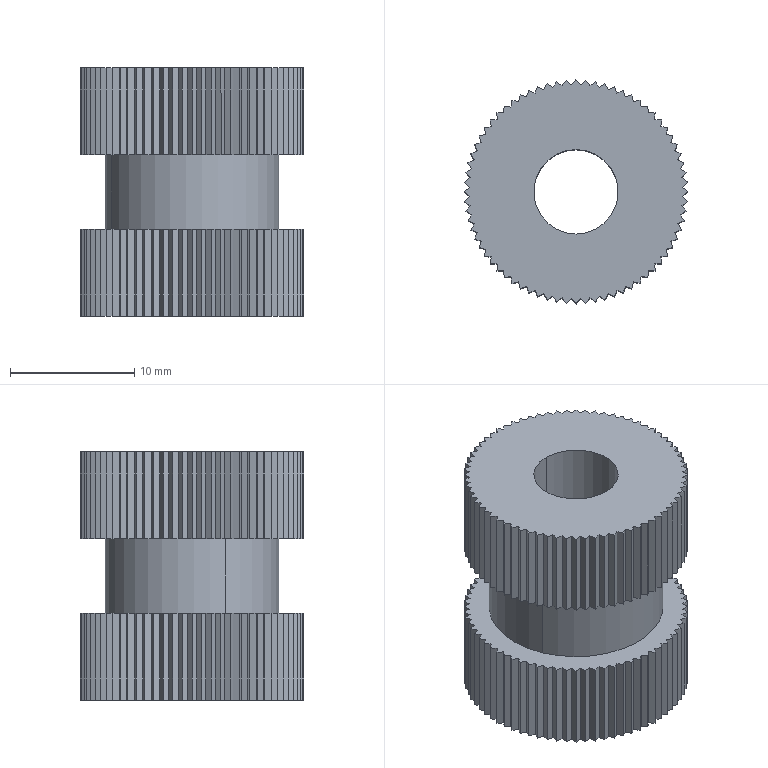Part | SolidWorks | features BaseBody 1 | 1 solid | 296 faces | box 18.005 x 18.005 x 20 mm | volume 3580 mm3 | plane 292 | cylinder 4 | commonest cylinder face diameters 6.8 x2 14 x2